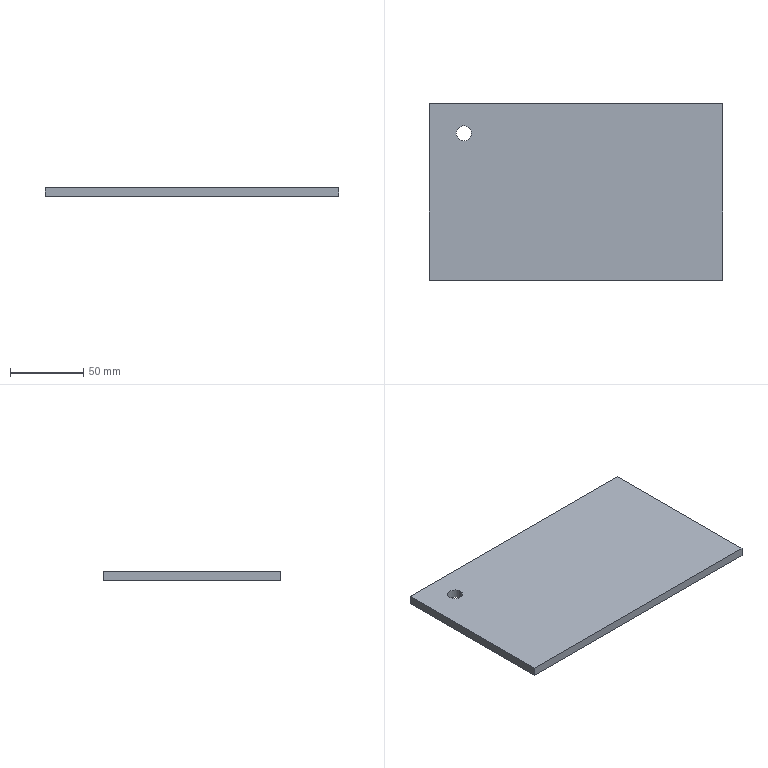Part | SolidWorks | features Extrusion 1, HoleWzd 1 | 1 solid | 8 faces | box 200 x 120 x 6 mm | volume 143510 mm3 | plane 6 | cylinder 2 | commonest cylinder face diameters 10.2 x2
STEP:
#1=CARTESIAN_POINT('',(-71.4,40.,0.));
#2=VERTEX_POINT('',#1);
#3=CARTESIAN_POINT('',(-81.6,40.,0.));
#4=VERTEX_POINT('',#3);
#5=CARTESIAN_POINT('',(-76.5,40.,0.));
#6=DIRECTION('',(0.,0.,-1.));
#7=DIRECTION('',(-1.,0.,0.));
#8=AXIS2_PLACEMENT_3D('',#5,#6,#7);
#9=CIRCLE('',#8,5.1);
#10=EDGE_CURVE('',#2,#4,#9,.T.);
#11=ORIENTED_EDGE('',*,*,#10,.T.);
#12=CARTESIAN_POINT('',(-81.6,40.,6.));
#13=VERTEX_POINT('',#12);
#14=CARTESIAN_POINT('',(-81.6,40.,6.));
#15=DIRECTION('',(0.,0.,1.));
#16=VECTOR('',#15,1000.);
#17=LINE('',#14,#16);
#18=EDGE_CURVE('',#4,#13,#17,.T.);
#19=ORIENTED_EDGE('',*,*,#18,.T.);
#20=CARTESIAN_POINT('',(-71.4,40.,6.));
#21=VERTEX_POINT('',#20);
#22=CARTESIAN_POINT('',(-76.5,40.,6.));
#23=DIRECTION('',(0.,0.,1.));
#24=DIRECTION('',(1.,0.,0.));
#25=AXIS2_PLACEMENT_3D('',#22,#23,#24);
#26=CIRCLE('',#25,5.1);
#27=EDGE_CURVE('',#13,#21,#26,.T.);
#28=ORIENTED_EDGE('',*,*,#27,.T.);
#29=CARTESIAN_POINT('',(-71.4,40.,6.));
#30=DIRECTION('',(0.,0.,1.));
#31=VECTOR('',#30,1000.);
#32=LINE('',#29,#31);
#33=EDGE_CURVE('',#2,#21,#32,.T.);
#34=ORIENTED_EDGE('',*,*,#33,.F.);
#35=EDGE_LOOP('',(#11,#19,#28,#34));
#36=FACE_OUTER_BOUND('',#35,.T.);
#37=CARTESIAN_POINT('',(-76.5,40.,6.));
#38=DIRECTION('',(0.,0.,1.));
#39=DIRECTION('',(1.,0.,0.));
#40=AXIS2_PLACEMENT_3D('',#37,#38,#39);
#41=CYLINDRICAL_SURFACE('',#40,5.1);
#42=ADVANCED_FACE('',(#36),#41,.F.);
#43=CARTESIAN_POINT('',(-100.,60.,0.));
#44=VERTEX_POINT('',#43);
#45=CARTESIAN_POINT('',(-100.,-60.,0.));
#46=VERTEX_POINT('',#45);
#47=CARTESIAN_POINT('',(-100.,60.,0.));
#48=DIRECTION('',(0.,-1.,0.));
#49=VECTOR('',#48,1000.);
#50=LINE('',#47,#49);
#51=EDGE_CURVE('',#44,#46,#50,.T.);
#52=ORIENTED_EDGE('',*,*,#51,.T.);
#53=CARTESIAN_POINT('',(-100.,-60.,6.));
#54=VERTEX_POINT('',#53);
#55=CARTESIAN_POINT('',(-100.,-60.,6.));
#56=DIRECTION('',(0.,0.,-1.));
#57=VECTOR('',#56,1000.);
#58=LINE('',#55,#57);
#59=EDGE_CURVE('',#54,#46,#58,.T.);
#60=ORIENTED_EDGE('',*,*,#59,.F.);
#61=CARTESIAN_POINT('',(-100.,60.,6.));
#62=VERTEX_POINT('',#61);
#63=CARTESIAN_POINT('',(-100.,60.,6.));
#64=DIRECTION('',(0.,-1.,0.));
#65=VECTOR('',#64,1000.);
#66=LINE('',#63,#65);
#67=EDGE_CURVE('',#62,#54,#66,.T.);
#68=ORIENTED_EDGE('',*,*,#67,.F.);
#69=CARTESIAN_POINT('',(-100.,60.,6.));
#70=DIRECTION('',(0.,0.,-1.));
#71=VECTOR('',#70,1000.);
#72=LINE('',#69,#71);
#73=EDGE_CURVE('',#62,#44,#72,.T.);
#74=ORIENTED_EDGE('',*,*,#73,.T.);
#75=EDGE_LOOP('',(#52,#60,#68,#74));
#76=FACE_OUTER_BOUND('',#75,.T.);
#77=CARTESIAN_POINT('',(-100.,60.,6.));
#78=DIRECTION('',(1.,0.,0.));
#79=DIRECTION('',(0.,1.,0.));
#80=AXIS2_PLACEMENT_3D('',#77,#78,#79);
#81=PLANE('',#80);
#82=ADVANCED_FACE('',(#76),#81,.F.);
#83=CARTESIAN_POINT('',(100.,-60.,0.));
#84=VERTEX_POINT('',#83);
#85=CARTESIAN_POINT('',(100.,-60.,0.));
#86=DIRECTION('',(1.,0.,0.));
#87=VECTOR('',#86,1000.);
#88=LINE('',#85,#87);
#89=EDGE_CURVE('',#46,#84,#88,.T.);
#90=ORIENTED_EDGE('',*,*,#89,.T.);
#91=CARTESIAN_POINT('',(100.,-60.,6.));
#92=VERTEX_POINT('',#91);
#93=CARTESIAN_POINT('',(100.,-60.,6.));
#94=DIRECTION('',(0.,0.,-1.));
#95=VECTOR('',#94,1000.);
#96=LINE('',#93,#95);
#97=EDGE_CURVE('',#92,#84,#96,.T.);
#98=ORIENTED_EDGE('',*,*,#97,.F.);
#99=CARTESIAN_POINT('',(100.,-60.,6.));
#100=DIRECTION('',(1.,0.,0.));
#101=VECTOR('',#100,1000.);
#102=LINE('',#99,#101);
#103=EDGE_CURVE('',#54,#92,#102,.T.);
#104=ORIENTED_EDGE('',*,*,#103,.F.);
#105=ORIENTED_EDGE('',*,*,#59,.T.);
#106=EDGE_LOOP('',(#90,#98,#104,#105));
#107=FACE_OUTER_BOUND('',#106,.T.);
#108=CARTESIAN_POINT('',(100.,-60.,6.));
#109=DIRECTION('',(0.,1.,0.));
#110=DIRECTION('',(-1.,0.,0.));
#111=AXIS2_PLACEMENT_3D('',#108,#109,#110);
#112=PLANE('',#111);
#113=ADVANCED_FACE('',(#107),#112,.F.);
#114=CARTESIAN_POINT('',(100.,60.,0.));
#115=VERTEX_POINT('',#114);
#116=CARTESIAN_POINT('',(100.,60.,0.));
#117=DIRECTION('',(0.,1.,0.));
#118=VECTOR('',#117,1000.);
#119=LINE('',#116,#118);
#120=EDGE_CURVE('',#84,#115,#119,.T.);
#121=ORIENTED_EDGE('',*,*,#120,.T.);
#122=CARTESIAN_POINT('',(100.,60.,6.));
#123=VERTEX_POINT('',#122);
#124=CARTESIAN_POINT('',(100.,60.,6.));
#125=DIRECTION('',(0.,0.,-1.));
#126=VECTOR('',#125,1000.);
#127=LINE('',#124,#126);
#128=EDGE_CURVE('',#123,#115,#127,.T.);
#129=ORIENTED_EDGE('',*,*,#128,.F.);
#130=CARTESIAN_POINT('',(100.,60.,6.));
#131=DIRECTION('',(0.,1.,0.));
#132=VECTOR('',#131,1000.);
#133=LINE('',#130,#132);
#134=EDGE_CURVE('',#92,#123,#133,.T.);
#135=ORIENTED_EDGE('',*,*,#134,.F.);
#136=ORIENTED_EDGE('',*,*,#97,.T.);
#137=EDGE_LOOP('',(#121,#129,#135,#136));
#138=FACE_OUTER_BOUND('',#137,.T.);
#139=CARTESIAN_POINT('',(100.,60.,6.));
#140=DIRECTION('',(-1.,0.,0.));
#141=DIRECTION('',(0.,-1.,0.));
#142=AXIS2_PLACEMENT_3D('',#139,#140,#141);
#143=PLANE('',#142);
#144=ADVANCED_FACE('',(#138),#143,.F.);
#145=CARTESIAN_POINT('',(100.,60.,0.));
#146=DIRECTION('',(-1.,0.,0.));
#147=VECTOR('',#146,1000.);
#148=LINE('',#145,#147);
#149=EDGE_CURVE('',#115,#44,#148,.T.);
#150=ORIENTED_EDGE('',*,*,#149,.T.);
#151=ORIENTED_EDGE('',*,*,#73,.F.);
#152=CARTESIAN_POINT('',(100.,60.,6.));
#153=DIRECTION('',(-1.,0.,0.));
#154=VECTOR('',#153,1000.);
#155=LINE('',#152,#154);
#156=EDGE_CURVE('',#123,#62,#155,.T.);
#157=ORIENTED_EDGE('',*,*,#156,.F.);
#158=ORIENTED_EDGE('',*,*,#128,.T.);
#159=EDGE_LOOP('',(#150,#151,#157,#158));
#160=FACE_OUTER_BOUND('',#159,.T.);
#161=CARTESIAN_POINT('',(100.,60.,6.));
#162=DIRECTION('',(0.,-1.,0.));
#163=DIRECTION('',(1.,0.,0.));
#164=AXIS2_PLACEMENT_3D('',#161,#162,#163);
#165=PLANE('',#164);
#166=ADVANCED_FACE('',(#160),#165,.F.);
#167=CARTESIAN_POINT('',(-76.5,40.,6.));
#168=DIRECTION('',(0.,0.,1.));
#169=DIRECTION('',(1.,0.,0.));
#170=AXIS2_PLACEMENT_3D('',#167,#168,#169);
#171=CIRCLE('',#170,5.1);
#172=EDGE_CURVE('',#21,#13,#171,.T.);
#173=ORIENTED_EDGE('',*,*,#172,.F.);
#174=ORIENTED_EDGE('',*,*,#27,.F.);
#175=EDGE_LOOP('',(#173,#174));
#176=FACE_BOUND('',#175,.T.);
#177=ORIENTED_EDGE('',*,*,#67,.T.);
#178=ORIENTED_EDGE('',*,*,#103,.T.);
#179=ORIENTED_EDGE('',*,*,#134,.T.);
#180=ORIENTED_EDGE('',*,*,#156,.T.);
#181=EDGE_LOOP('',(#177,#178,#179,#180));
#182=FACE_OUTER_BOUND('',#181,.T.);
#183=CARTESIAN_POINT('',(0.,0.,6.));
#184=DIRECTION('',(0.,0.,-1.));
#185=DIRECTION('',(-1.,0.,0.));
#186=AXIS2_PLACEMENT_3D('',#183,#184,#185);
#187=PLANE('',#186);
#188=ADVANCED_FACE('',(#176,#182),#187,.F.);
#189=ORIENTED_EDGE('',*,*,#10,.F.);
#190=CARTESIAN_POINT('',(-76.5,40.,0.));
#191=DIRECTION('',(0.,0.,-1.));
#192=DIRECTION('',(-1.,0.,0.));
#193=AXIS2_PLACEMENT_3D('',#190,#191,#192);
#194=CIRCLE('',#193,5.1);
#195=EDGE_CURVE('',#4,#2,#194,.T.);
#196=ORIENTED_EDGE('',*,*,#195,.F.);
#197=EDGE_LOOP('',(#189,#196));
#198=FACE_BOUND('',#197,.T.);
#199=ORIENTED_EDGE('',*,*,#51,.F.);
#200=ORIENTED_EDGE('',*,*,#149,.F.);
#201=ORIENTED_EDGE('',*,*,#120,.F.);
#202=ORIENTED_EDGE('',*,*,#89,.F.);
#203=EDGE_LOOP('',(#199,#200,#201,#202));
#204=FACE_OUTER_BOUND('',#203,.T.);
#205=CARTESIAN_POINT('',(0.,0.,0.));
#206=DIRECTION('',(0.,0.,-1.));
#207=DIRECTION('',(-1.,0.,0.));
#208=AXIS2_PLACEMENT_3D('',#205,#206,#207);
#209=PLANE('',#208);
#210=ADVANCED_FACE('',(#198,#204),#209,.T.);
#211=ORIENTED_EDGE('',*,*,#18,.F.);
#212=ORIENTED_EDGE('',*,*,#195,.T.);
#213=ORIENTED_EDGE('',*,*,#33,.T.);
#214=ORIENTED_EDGE('',*,*,#172,.T.);
#215=EDGE_LOOP('',(#211,#212,#213,#214));
#216=FACE_OUTER_BOUND('',#215,.T.);
#217=CARTESIAN_POINT('',(-76.5,40.,6.));
#218=DIRECTION('',(0.,0.,1.));
#219=DIRECTION('',(1.,0.,0.));
#220=AXIS2_PLACEMENT_3D('',#217,#218,#219);
#221=CYLINDRICAL_SURFACE('',#220,5.1);
#222=ADVANCED_FACE('',(#216),#221,.F.);
#223=CLOSED_SHELL('',(#42,#82,#113,#144,#166,#188,#210,#222));
#224=MANIFOLD_SOLID_BREP('',#223);
#225=CARTESIAN_POINT('',(0.,0.,0.));
#226=DIRECTION('',(0.,0.,1.));
#227=DIRECTION('',(1.,0.,0.));
#228=AXIS2_PLACEMENT_3D('',#225,#226,#227);
#229=(LENGTH_UNIT()NAMED_UNIT(*)SI_UNIT(.MILLI.,.METRE.));
#230=UNCERTAINTY_MEASURE_WITH_UNIT(LENGTH_MEASURE(0.00001),#229,'','');
#231=(NAMED_UNIT(*)PLANE_ANGLE_UNIT()SI_UNIT($,.RADIAN.));
#232=(NAMED_UNIT(*)SI_UNIT($,.STERADIAN.)SOLID_ANGLE_UNIT());
#233=(GEOMETRIC_REPRESENTATION_CONTEXT(3)GLOBAL_UNCERTAINTY_ASSIGNED_CONTEXT((#230))GLOBAL_UNIT_ASSIGNED_CONTEXT((#229,#231,#232))REPRESENTATION_CONTEXT('',''));
#234=ADVANCED_BREP_SHAPE_REPRESENTATION('',(#224,#228),#233);